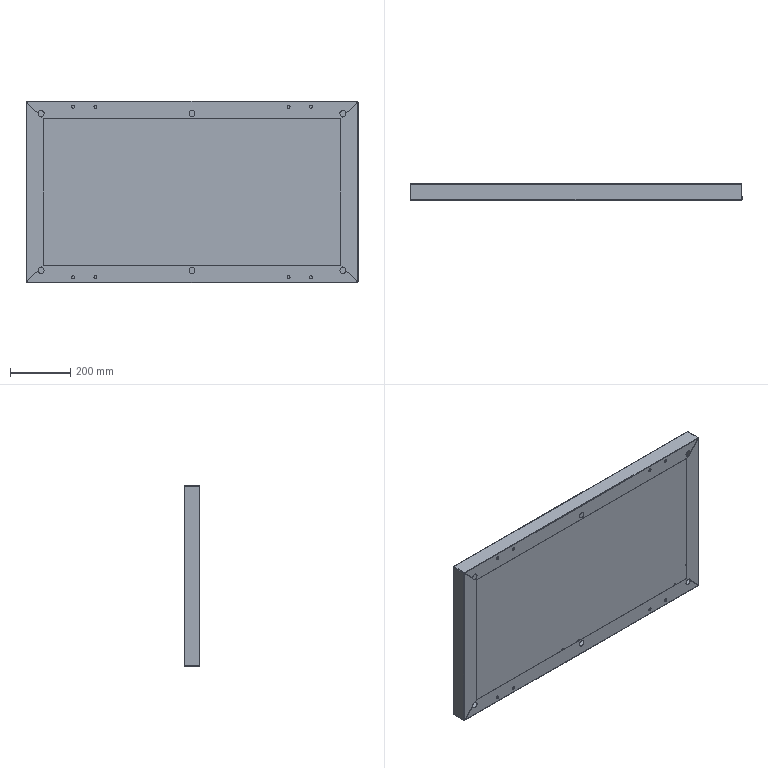Part | SolidWorks | features SplitBody 1 | 1 solid | 128 faces | box 1100 x 53 x 600.001 mm | volume 1504531 mm3 | cylinder 66 | plane 46 | spline 16 | commonest cylinder face diameters 4.5 x20 10 x16 20 x14 0.2 x8 3.2 x8